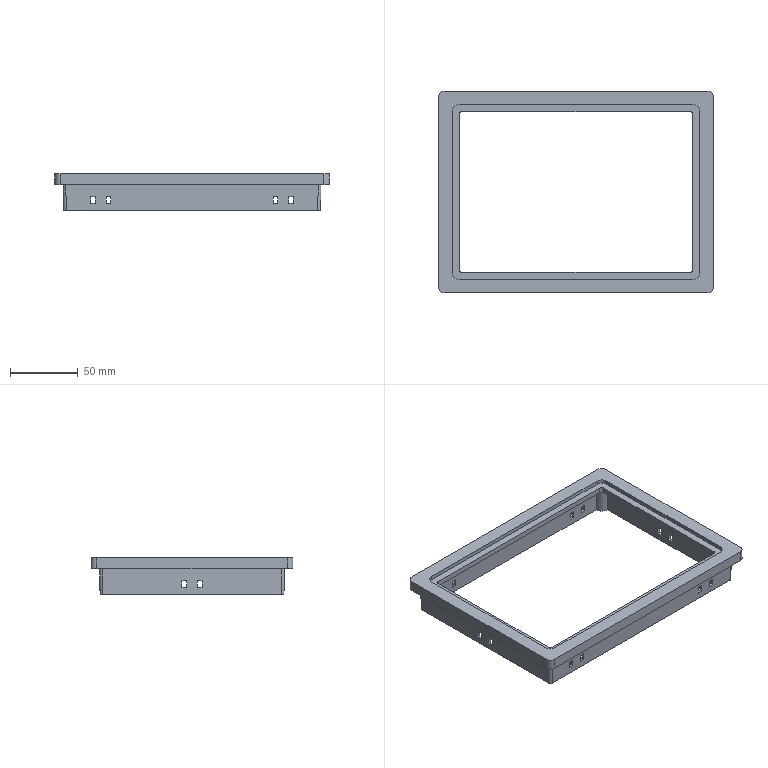Part | SolidWorks | features BaseBody 1 | 1 solid | 132 faces | box 203 x 149 x 27 mm | volume 76480 mm3 | plane 92 | cylinder 40 | commonest cylinder face diameters 3 x12 4 x8 2 x4 6 x4 8 x4 10 x4